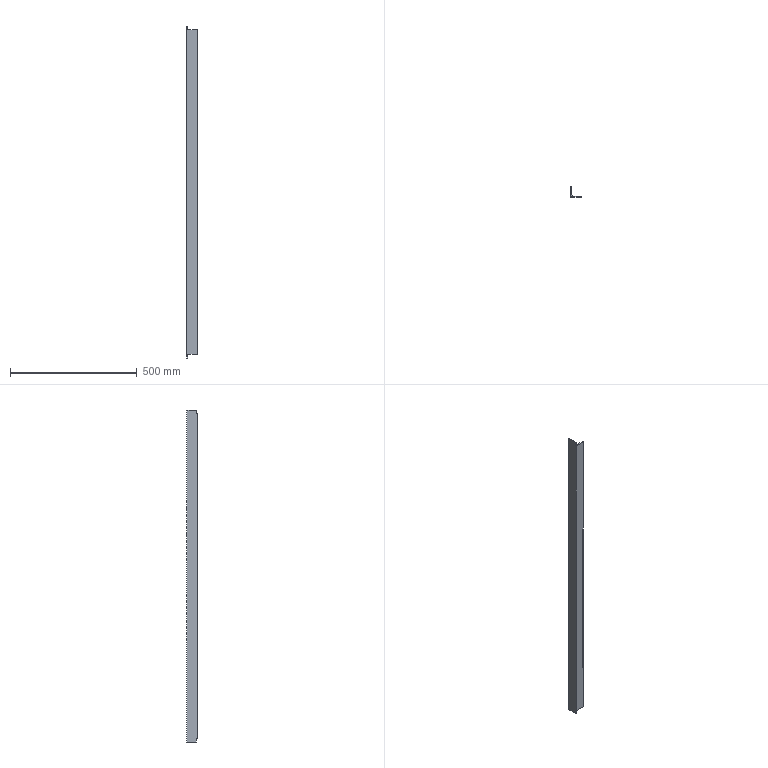Part | SolidWorks | features BaseBody 1 | 1 solid | 13 faces | box 40 x 40 x 1310 mm | volume 299570 mm3 | plane 10 | cylinder 3 | commonest cylinder face diameters 6 x2 9 x1
STEP:
#1=CARTESIAN_POINT('',(0.,3.,1335.));
#2=VERTEX_POINT('',#1);
#3=CARTESIAN_POINT('',(3.,3.,1335.));
#4=VERTEX_POINT('',#3);
#5=CARTESIAN_POINT('',(-7.,3.,1335.));
#6=DIRECTION('',(1.,0.,0.));
#7=VECTOR('',#6,1000.);
#8=LINE('',#5,#7);
#9=EDGE_CURVE('',#2,#4,#8,.T.);
#10=ORIENTED_EDGE('',*,*,#9,.T.);
#11=CARTESIAN_POINT('',(3.,37.,1335.));
#12=VERTEX_POINT('',#11);
#13=CARTESIAN_POINT('',(3.,3.,1335.));
#14=DIRECTION('',(0.,1.,0.));
#15=VECTOR('',#14,1000.);
#16=LINE('',#13,#15);
#17=EDGE_CURVE('',#4,#12,#16,.T.);
#18=ORIENTED_EDGE('',*,*,#17,.T.);
#19=CARTESIAN_POINT('',(0.,40.,1335.));
#20=VERTEX_POINT('',#19);
#21=CARTESIAN_POINT('',(0.,37.,1335.));
#22=DIRECTION('',(0.,0.,1.));
#23=DIRECTION('',(-1.,0.,0.));
#24=AXIS2_PLACEMENT_3D('',#21,#22,#23);
#25=CIRCLE('',#24,3.);
#26=EDGE_CURVE('',#12,#20,#25,.T.);
#27=ORIENTED_EDGE('',*,*,#26,.T.);
#28=CARTESIAN_POINT('',(0.,0.,1335.));
#29=DIRECTION('',(0.,1.,0.));
#30=VECTOR('',#29,1000.);
#31=LINE('',#28,#30);
#32=EDGE_CURVE('',#2,#20,#31,.T.);
#33=ORIENTED_EDGE('',*,*,#32,.F.);
#34=EDGE_LOOP('',(#10,#18,#27,#33));
#35=FACE_OUTER_BOUND('',#34,.T.);
#36=CARTESIAN_POINT('',(-7.,3.,1335.));
#37=DIRECTION('',(0.,0.,-1.));
#38=DIRECTION('',(0.,-1.,0.));
#39=AXIS2_PLACEMENT_3D('',#36,#37,#38);
#40=PLANE('',#39);
#41=ADVANCED_FACE('',(#35),#40,.F.);
#42=CARTESIAN_POINT('',(0.,40.,25.));
#43=VERTEX_POINT('',#42);
#44=CARTESIAN_POINT('',(3.,37.,25.));
#45=VERTEX_POINT('',#44);
#46=CARTESIAN_POINT('',(0.,37.,25.));
#47=DIRECTION('',(0.,0.,-1.));
#48=DIRECTION('',(1.,0.,0.));
#49=AXIS2_PLACEMENT_3D('',#46,#47,#48);
#50=CIRCLE('',#49,3.);
#51=EDGE_CURVE('',#43,#45,#50,.T.);
#52=ORIENTED_EDGE('',*,*,#51,.T.);
#53=CARTESIAN_POINT('',(3.,3.,25.));
#54=VERTEX_POINT('',#53);
#55=CARTESIAN_POINT('',(3.,3.,25.));
#56=DIRECTION('',(0.,-1.,0.));
#57=VECTOR('',#56,1000.);
#58=LINE('',#55,#57);
#59=EDGE_CURVE('',#45,#54,#58,.T.);
#60=ORIENTED_EDGE('',*,*,#59,.T.);
#61=CARTESIAN_POINT('',(0.,3.,25.));
#62=VERTEX_POINT('',#61);
#63=CARTESIAN_POINT('',(0.,3.,25.));
#64=DIRECTION('',(1.,0.,0.));
#65=VECTOR('',#64,1000.);
#66=LINE('',#63,#65);
#67=EDGE_CURVE('',#62,#54,#66,.T.);
#68=ORIENTED_EDGE('',*,*,#67,.F.);
#69=CARTESIAN_POINT('',(0.,0.,25.));
#70=DIRECTION('',(0.,-1.,0.));
#71=VECTOR('',#70,1000.);
#72=LINE('',#69,#71);
#73=EDGE_CURVE('',#43,#62,#72,.T.);
#74=ORIENTED_EDGE('',*,*,#73,.F.);
#75=EDGE_LOOP('',(#52,#60,#68,#74));
#76=FACE_OUTER_BOUND('',#75,.T.);
#77=CARTESIAN_POINT('',(-7.,3.,25.));
#78=DIRECTION('',(0.,0.,1.));
#79=DIRECTION('',(1.,0.,0.));
#80=AXIS2_PLACEMENT_3D('',#77,#78,#79);
#81=PLANE('',#80);
#82=ADVANCED_FACE('',(#76),#81,.F.);
#83=CARTESIAN_POINT('',(40.,0.,1320.));
#84=VERTEX_POINT('',#83);
#85=CARTESIAN_POINT('',(37.,3.,1320.));
#86=VERTEX_POINT('',#85);
#87=CARTESIAN_POINT('',(37.,0.,1320.));
#88=DIRECTION('',(0.,0.,1.));
#89=DIRECTION('',(-1.,0.,0.));
#90=AXIS2_PLACEMENT_3D('',#87,#88,#89);
#91=CIRCLE('',#90,3.);
#92=EDGE_CURVE('',#84,#86,#91,.T.);
#93=ORIENTED_EDGE('',*,*,#92,.T.);
#94=CARTESIAN_POINT('',(7.5,3.,1320.));
#95=VERTEX_POINT('',#94);
#96=CARTESIAN_POINT('',(0.,3.,1320.));
#97=DIRECTION('',(1.,0.,0.));
#98=VECTOR('',#97,1000.);
#99=LINE('',#96,#98);
#100=EDGE_CURVE('',#95,#86,#99,.T.);
#101=ORIENTED_EDGE('',*,*,#100,.F.);
#102=CARTESIAN_POINT('',(3.,7.5,1320.));
#103=VERTEX_POINT('',#102);
#104=CARTESIAN_POINT('',(7.5,7.5,1320.));
#105=DIRECTION('',(0.,0.,-1.));
#106=DIRECTION('',(1.,0.,0.));
#107=AXIS2_PLACEMENT_3D('',#104,#105,#106);
#108=CIRCLE('',#107,4.5);
#109=EDGE_CURVE('',#95,#103,#108,.T.);
#110=ORIENTED_EDGE('',*,*,#109,.T.);
#111=CARTESIAN_POINT('',(3.,3.,1320.));
#112=VERTEX_POINT('',#111);
#113=CARTESIAN_POINT('',(3.,0.,1320.));
#114=DIRECTION('',(0.,1.,0.));
#115=VECTOR('',#114,1000.);
#116=LINE('',#113,#115);
#117=EDGE_CURVE('',#112,#103,#116,.T.);
#118=ORIENTED_EDGE('',*,*,#117,.F.);
#119=CARTESIAN_POINT('',(0.,3.,1320.));
#120=VERTEX_POINT('',#119);
#121=CARTESIAN_POINT('',(0.,3.,1320.));
#122=DIRECTION('',(1.,0.,0.));
#123=VECTOR('',#122,1000.);
#124=LINE('',#121,#123);
#125=EDGE_CURVE('',#120,#112,#124,.T.);
#126=ORIENTED_EDGE('',*,*,#125,.F.);
#127=CARTESIAN_POINT('',(0.,0.,1320.));
#128=VERTEX_POINT('',#127);
#129=CARTESIAN_POINT('',(0.,3.,1320.));
#130=DIRECTION('',(0.,-1.,0.));
#131=VECTOR('',#130,1000.);
#132=LINE('',#129,#131);
#133=EDGE_CURVE('',#120,#128,#132,.T.);
#134=ORIENTED_EDGE('',*,*,#133,.T.);
#135=CARTESIAN_POINT('',(0.,0.,1320.));
#136=DIRECTION('',(1.,0.,0.));
#137=VECTOR('',#136,1000.);
#138=LINE('',#135,#137);
#139=EDGE_CURVE('',#128,#84,#138,.T.);
#140=ORIENTED_EDGE('',*,*,#139,.T.);
#141=EDGE_LOOP('',(#93,#101,#110,#118,#126,#134,#140));
#142=FACE_OUTER_BOUND('',#141,.T.);
#143=CARTESIAN_POINT('',(0.,3.,1320.));
#144=DIRECTION('',(0.,0.,-1.));
#145=DIRECTION('',(0.,-1.,0.));
#146=AXIS2_PLACEMENT_3D('',#143,#144,#145);
#147=PLANE('',#146);
#148=ADVANCED_FACE('',(#142),#147,.F.);
#149=CARTESIAN_POINT('',(37.,3.,40.));
#150=VERTEX_POINT('',#149);
#151=CARTESIAN_POINT('',(40.,0.,40.));
#152=VERTEX_POINT('',#151);
#153=CARTESIAN_POINT('',(37.,0.,40.));
#154=DIRECTION('',(0.,0.,-1.));
#155=DIRECTION('',(1.,0.,0.));
#156=AXIS2_PLACEMENT_3D('',#153,#154,#155);
#157=CIRCLE('',#156,3.);
#158=EDGE_CURVE('',#150,#152,#157,.T.);
#159=ORIENTED_EDGE('',*,*,#158,.T.);
#160=CARTESIAN_POINT('',(0.,0.,40.));
#161=VERTEX_POINT('',#160);
#162=CARTESIAN_POINT('',(0.,0.,40.));
#163=DIRECTION('',(-1.,0.,0.));
#164=VECTOR('',#163,1000.);
#165=LINE('',#162,#164);
#166=EDGE_CURVE('',#152,#161,#165,.T.);
#167=ORIENTED_EDGE('',*,*,#166,.T.);
#168=CARTESIAN_POINT('',(0.,3.,40.));
#169=VERTEX_POINT('',#168);
#170=CARTESIAN_POINT('',(0.,3.,40.));
#171=DIRECTION('',(0.,-1.,0.));
#172=VECTOR('',#171,1000.);
#173=LINE('',#170,#172);
#174=EDGE_CURVE('',#169,#161,#173,.T.);
#175=ORIENTED_EDGE('',*,*,#174,.F.);
#176=CARTESIAN_POINT('',(3.,3.,40.));
#177=VERTEX_POINT('',#176);
#178=CARTESIAN_POINT('',(0.,3.,40.));
#179=DIRECTION('',(-1.,0.,0.));
#180=VECTOR('',#179,1000.);
#181=LINE('',#178,#180);
#182=EDGE_CURVE('',#177,#169,#181,.T.);
#183=ORIENTED_EDGE('',*,*,#182,.F.);
#184=CARTESIAN_POINT('',(3.,7.5,40.));
#185=VERTEX_POINT('',#184);
#186=CARTESIAN_POINT('',(3.,3.,40.));
#187=DIRECTION('',(0.,-1.,0.));
#188=VECTOR('',#187,1000.);
#189=LINE('',#186,#188);
#190=EDGE_CURVE('',#185,#177,#189,.T.);
#191=ORIENTED_EDGE('',*,*,#190,.F.);
#192=CARTESIAN_POINT('',(7.5,3.,40.));
#193=VERTEX_POINT('',#192);
#194=CARTESIAN_POINT('',(7.5,7.5,40.));
#195=DIRECTION('',(0.,0.,1.));
#196=DIRECTION('',(-1.,0.,0.));
#197=AXIS2_PLACEMENT_3D('',#194,#195,#196);
#198=CIRCLE('',#197,4.5);
#199=EDGE_CURVE('',#185,#193,#198,.T.);
#200=ORIENTED_EDGE('',*,*,#199,.T.);
#201=CARTESIAN_POINT('',(0.,3.,40.));
#202=DIRECTION('',(-1.,0.,0.));
#203=VECTOR('',#202,1000.);
#204=LINE('',#201,#203);
#205=EDGE_CURVE('',#150,#193,#204,.T.);
#206=ORIENTED_EDGE('',*,*,#205,.F.);
#207=EDGE_LOOP('',(#159,#167,#175,#183,#191,#200,#206));
#208=FACE_OUTER_BOUND('',#207,.T.);
#209=CARTESIAN_POINT('',(0.,3.,40.));
#210=DIRECTION('',(0.,0.,1.));
#211=DIRECTION('',(1.,0.,0.));
#212=AXIS2_PLACEMENT_3D('',#209,#210,#211);
#213=PLANE('',#212);
#214=ADVANCED_FACE('',(#208),#213,.F.);
#215=CARTESIAN_POINT('',(0.,3.,0.));
#216=DIRECTION('',(0.,0.,-1.));
#217=VECTOR('',#216,1000.);
#218=LINE('',#215,#217);
#219=EDGE_CURVE('',#169,#62,#218,.T.);
#220=ORIENTED_EDGE('',*,*,#219,.T.);
#221=ORIENTED_EDGE('',*,*,#67,.T.);
#222=CARTESIAN_POINT('',(3.,3.,40.));
#223=DIRECTION('',(0.,0.,-1.));
#224=VECTOR('',#223,1000.);
#225=LINE('',#222,#224);
#226=EDGE_CURVE('',#177,#54,#225,.T.);
#227=ORIENTED_EDGE('',*,*,#226,.F.);
#228=ORIENTED_EDGE('',*,*,#182,.T.);
#229=EDGE_LOOP('',(#220,#221,#227,#228));
#230=FACE_OUTER_BOUND('',#229,.T.);
#231=CARTESIAN_POINT('',(0.,3.,0.));
#232=DIRECTION('',(0.,1.,0.));
#233=DIRECTION('',(1.,0.,0.));
#234=AXIS2_PLACEMENT_3D('',#231,#232,#233);
#235=PLANE('',#234);
#236=ADVANCED_FACE('',(#230),#235,.F.);
#237=ORIENTED_EDGE('',*,*,#26,.F.);
#238=CARTESIAN_POINT('',(3.,37.,1360.));
#239=DIRECTION('',(0.,0.,1.));
#240=VECTOR('',#239,1000.);
#241=LINE('',#238,#240);
#242=EDGE_CURVE('',#45,#12,#241,.T.);
#243=ORIENTED_EDGE('',*,*,#242,.F.);
#244=ORIENTED_EDGE('',*,*,#51,.F.);
#245=CARTESIAN_POINT('',(0.,40.,1360.));
#246=DIRECTION('',(0.,0.,-1.));
#247=VECTOR('',#246,1000.);
#248=LINE('',#245,#247);
#249=EDGE_CURVE('',#20,#43,#248,.T.);
#250=ORIENTED_EDGE('',*,*,#249,.F.);
#251=EDGE_LOOP('',(#237,#243,#244,#250));
#252=FACE_OUTER_BOUND('',#251,.T.);
#253=CARTESIAN_POINT('',(0.,37.,1360.));
#254=DIRECTION('',(0.,0.,-1.));
#255=DIRECTION('',(-1.,0.,0.));
#256=AXIS2_PLACEMENT_3D('',#253,#254,#255);
#257=CYLINDRICAL_SURFACE('',#256,3.);
#258=ADVANCED_FACE('',(#252),#257,.T.);
#259=ORIENTED_EDGE('',*,*,#92,.F.);
#260=CARTESIAN_POINT('',(40.,0.,1360.));
#261=DIRECTION('',(0.,0.,-1.));
#262=VECTOR('',#261,1000.);
#263=LINE('',#260,#262);
#264=EDGE_CURVE('',#84,#152,#263,.T.);
#265=ORIENTED_EDGE('',*,*,#264,.T.);
#266=ORIENTED_EDGE('',*,*,#158,.F.);
#267=CARTESIAN_POINT('',(37.,3.,1360.));
#268=DIRECTION('',(0.,0.,-1.));
#269=VECTOR('',#268,1000.);
#270=LINE('',#267,#269);
#271=EDGE_CURVE('',#86,#150,#270,.T.);
#272=ORIENTED_EDGE('',*,*,#271,.F.);
#273=EDGE_LOOP('',(#259,#265,#266,#272));
#274=FACE_OUTER_BOUND('',#273,.T.);
#275=CARTESIAN_POINT('',(37.,0.,1360.));
#276=DIRECTION('',(0.,0.,-1.));
#277=DIRECTION('',(-1.,0.,0.));
#278=AXIS2_PLACEMENT_3D('',#275,#276,#277);
#279=CYLINDRICAL_SURFACE('',#278,3.);
#280=ADVANCED_FACE('',(#274),#279,.T.);
#281=ORIENTED_EDGE('',*,*,#242,.T.);
#282=ORIENTED_EDGE('',*,*,#17,.F.);
#283=CARTESIAN_POINT('',(3.,3.,0.));
#284=DIRECTION('',(0.,0.,1.));
#285=VECTOR('',#284,1000.);
#286=LINE('',#283,#285);
#287=EDGE_CURVE('',#112,#4,#286,.T.);
#288=ORIENTED_EDGE('',*,*,#287,.F.);
#289=ORIENTED_EDGE('',*,*,#117,.T.);
#290=CARTESIAN_POINT('',(3.,7.5,0.));
#291=DIRECTION('',(0.,0.,-1.));
#292=VECTOR('',#291,1000.);
#293=LINE('',#290,#292);
#294=EDGE_CURVE('',#103,#185,#293,.T.);
#295=ORIENTED_EDGE('',*,*,#294,.T.);
#296=ORIENTED_EDGE('',*,*,#190,.T.);
#297=ORIENTED_EDGE('',*,*,#226,.T.);
#298=ORIENTED_EDGE('',*,*,#59,.F.);
#299=EDGE_LOOP('',(#281,#282,#288,#289,#295,#296,#297,#298));
#300=FACE_OUTER_BOUND('',#299,.T.);
#301=CARTESIAN_POINT('',(3.,40.,1360.));
#302=DIRECTION('',(-1.,0.,0.));
#303=DIRECTION('',(0.,1.,0.));
#304=AXIS2_PLACEMENT_3D('',#301,#302,#303);
#305=PLANE('',#304);
#306=ADVANCED_FACE('',(#300),#305,.F.);
#307=CARTESIAN_POINT('',(7.5,3.,1360.));
#308=DIRECTION('',(0.,0.,1.));
#309=VECTOR('',#308,1000.);
#310=LINE('',#307,#309);
#311=EDGE_CURVE('',#193,#95,#310,.T.);
#312=ORIENTED_EDGE('',*,*,#311,.T.);
#313=ORIENTED_EDGE('',*,*,#100,.T.);
#314=ORIENTED_EDGE('',*,*,#271,.T.);
#315=ORIENTED_EDGE('',*,*,#205,.T.);
#316=EDGE_LOOP('',(#312,#313,#314,#315));
#317=FACE_OUTER_BOUND('',#316,.T.);
#318=CARTESIAN_POINT('',(3.,3.,1360.));
#319=DIRECTION('',(0.,-1.,0.));
#320=DIRECTION('',(0.,0.,-1.));
#321=AXIS2_PLACEMENT_3D('',#318,#319,#320);
#322=PLANE('',#321);
#323=ADVANCED_FACE('',(#317),#322,.F.);
#324=ORIENTED_EDGE('',*,*,#264,.F.);
#325=ORIENTED_EDGE('',*,*,#139,.F.);
#326=CARTESIAN_POINT('',(0.,0.,1360.));
#327=DIRECTION('',(0.,0.,-1.));
#328=VECTOR('',#327,1000.);
#329=LINE('',#326,#328);
#330=EDGE_CURVE('',#128,#161,#329,.T.);
#331=ORIENTED_EDGE('',*,*,#330,.T.);
#332=ORIENTED_EDGE('',*,*,#166,.F.);
#333=EDGE_LOOP('',(#324,#325,#331,#332));
#334=FACE_OUTER_BOUND('',#333,.T.);
#335=CARTESIAN_POINT('',(0.,0.,1360.));
#336=DIRECTION('',(0.,1.,0.));
#337=DIRECTION('',(1.,0.,0.));
#338=AXIS2_PLACEMENT_3D('',#335,#336,#337);
#339=PLANE('',#338);
#340=ADVANCED_FACE('',(#334),#339,.F.);
#341=CARTESIAN_POINT('',(0.,3.,1360.));
#342=DIRECTION('',(0.,0.,-1.));
#343=VECTOR('',#342,1000.);
#344=LINE('',#341,#343);
#345=EDGE_CURVE('',#2,#120,#344,.T.);
#346=ORIENTED_EDGE('',*,*,#345,.F.);
#347=ORIENTED_EDGE('',*,*,#32,.T.);
#348=ORIENTED_EDGE('',*,*,#249,.T.);
#349=ORIENTED_EDGE('',*,*,#73,.T.);
#350=ORIENTED_EDGE('',*,*,#219,.F.);
#351=ORIENTED_EDGE('',*,*,#174,.T.);
#352=ORIENTED_EDGE('',*,*,#330,.F.);
#353=ORIENTED_EDGE('',*,*,#133,.F.);
#354=EDGE_LOOP('',(#346,#347,#348,#349,#350,#351,#352,#353));
#355=FACE_OUTER_BOUND('',#354,.T.);
#356=CARTESIAN_POINT('',(0.,0.,1360.));
#357=DIRECTION('',(1.,0.,0.));
#358=DIRECTION('',(0.,1.,0.));
#359=AXIS2_PLACEMENT_3D('',#356,#357,#358);
#360=PLANE('',#359);
#361=ADVANCED_FACE('',(#355),#360,.F.);
#362=ORIENTED_EDGE('',*,*,#9,.F.);
#363=ORIENTED_EDGE('',*,*,#345,.T.);
#364=ORIENTED_EDGE('',*,*,#125,.T.);
#365=ORIENTED_EDGE('',*,*,#287,.T.);
#366=EDGE_LOOP('',(#362,#363,#364,#365));
#367=FACE_OUTER_BOUND('',#366,.T.);
#368=CARTESIAN_POINT('',(0.,3.,0.));
#369=DIRECTION('',(0.,-1.,0.));
#370=DIRECTION('',(0.,0.,-1.));
#371=AXIS2_PLACEMENT_3D('',#368,#369,#370);
#372=PLANE('',#371);
#373=ADVANCED_FACE('',(#367),#372,.T.);
#374=ORIENTED_EDGE('',*,*,#109,.F.);
#375=ORIENTED_EDGE('',*,*,#311,.F.);
#376=ORIENTED_EDGE('',*,*,#199,.F.);
#377=ORIENTED_EDGE('',*,*,#294,.F.);
#378=EDGE_LOOP('',(#374,#375,#376,#377));
#379=FACE_OUTER_BOUND('',#378,.T.);
#380=CARTESIAN_POINT('',(7.5,7.5,1360.));
#381=DIRECTION('',(0.,0.,1.));
#382=DIRECTION('',(1.,0.,0.));
#383=AXIS2_PLACEMENT_3D('',#380,#381,#382);
#384=CYLINDRICAL_SURFACE('',#383,4.5);
#385=ADVANCED_FACE('',(#379),#384,.F.);
#386=CLOSED_SHELL('',(#41,#82,#148,#214,#236,#258,#280,#306,#323,#340,#361,#373,#385));
#387=MANIFOLD_SOLID_BREP('',#386);
#388=CARTESIAN_POINT('',(0.,0.,0.));
#389=DIRECTION('',(0.,0.,1.));
#390=DIRECTION('',(1.,0.,0.));
#391=AXIS2_PLACEMENT_3D('',#388,#389,#390);
#392=(LENGTH_UNIT()NAMED_UNIT(*)SI_UNIT(.MILLI.,.METRE.));
#393=UNCERTAINTY_MEASURE_WITH_UNIT(LENGTH_MEASURE(0.00001),#392,'','');
#394=(NAMED_UNIT(*)PLANE_ANGLE_UNIT()SI_UNIT($,.RADIAN.));
#395=(NAMED_UNIT(*)SI_UNIT($,.STERADIAN.)SOLID_ANGLE_UNIT());
#396=(GEOMETRIC_REPRESENTATION_CONTEXT(3)GLOBAL_UNCERTAINTY_ASSIGNED_CONTEXT((#393))GLOBAL_UNIT_ASSIGNED_CONTEXT((#392,#394,#395))REPRESENTATION_CONTEXT('',''));
#397=ADVANCED_BREP_SHAPE_REPRESENTATION('',(#387,#391),#396);